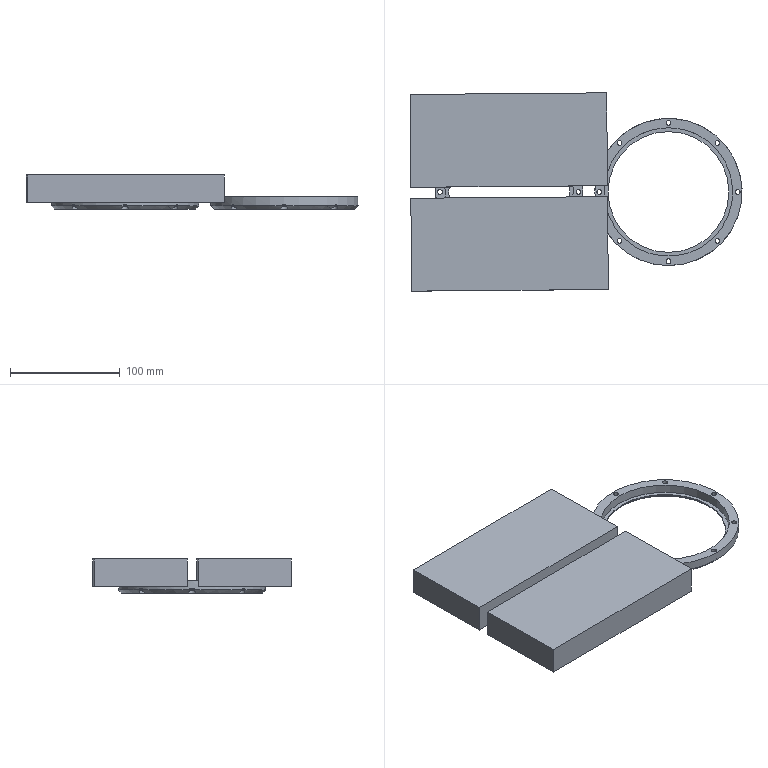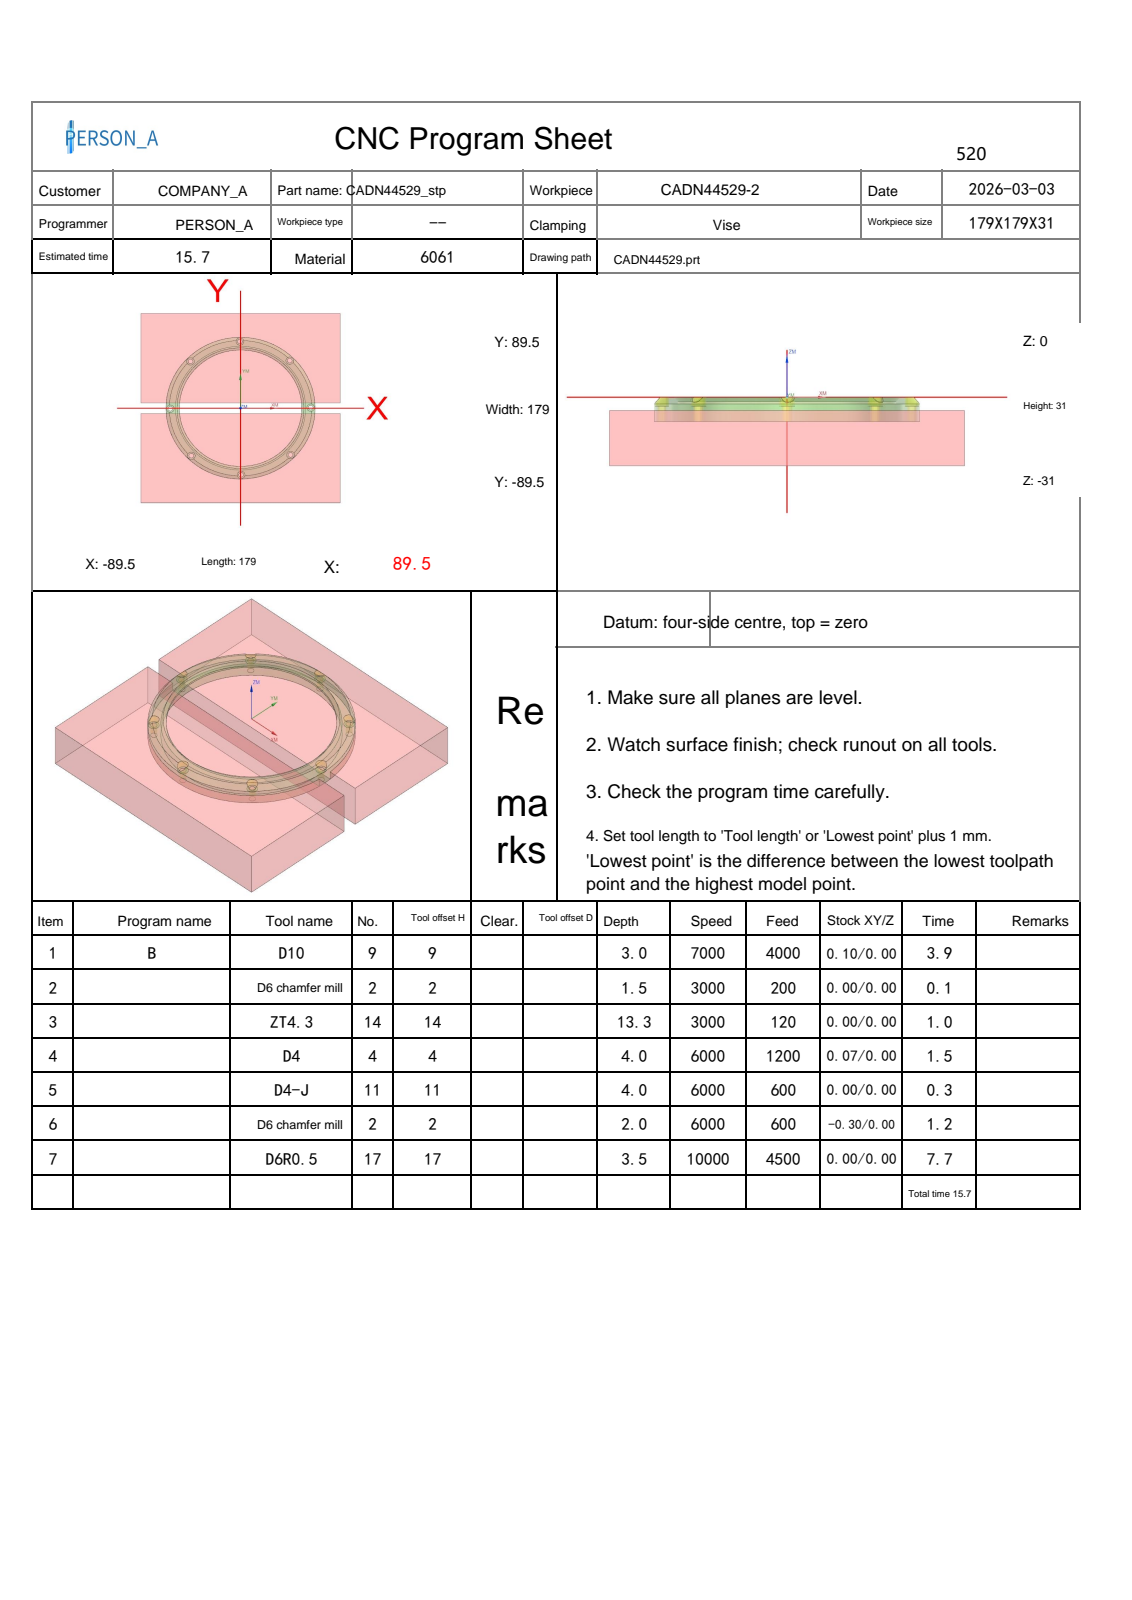NC program | NX | posted by the shop | part box 302.234 x 180.468 x 31 mm
Lines 21303 to 22985 of 75694, first 1471 of 1683 lines:
N2 T02 M06
(D6 chamfer mill  D=6. R=0. H=02 ce=0.00 di=0.00)
G00 G90 G54 X-44.913 Y44.179 M03 S3000
G43 H02 Z50.
M08
G98 G81 X-44.913 Y44.179 Z-1.5 R1. F200.
X-62.998 Y-.519
X-44.179 Y-44.913
X.519 Y-62.998
X44.913 Y-44.179
X62.998 Y.519
X44.179 Y44.913
X-.519 Y62.998
G80
G00 Z50.
G91 G28 Z0.0
M05
M09
G91 G28 Z0.0
M01
N3 T14 M06
(ZT4.3 D=4.3 DR_a=118 H=14)
G00 G90 G54 X-44.913 Y44.179 M03 S3000
G43 H14 Z50.
M08
G98 G83 X-44.913 Y44.179 Z-13.292 R1. F120. Q3.
X-62.998 Y-.519
X-44.179 Y-44.913
X.519 Y-62.998
X44.913 Y-44.179
X62.998 Y.519
X44.179 Y44.913
X-.519 Y62.998
G80
G00 Z50.
G91 G28 Z0.0
M05
M09
G91 G28 Z0.0
M01
N4 T04 M06
(D4  D=4. R=0. H=04 ce=0.07 di=0.00)
G00 G90 G54 X44.179 Y44.913 M03 S6000
G43 H04 Z50.
M08
Z.3
G03 X44.894 Y44.204 I.715 J.006 F1200.
X45.609 Y44.919 I0.0 J.715
G01 Y44.925
G03 X45.609 Y44.925 Z.1 I-1.43 J-.012
X45.609 Y44.925 Z-.1 I-1.43 J-.012
X45.609 Y44.925 Z-.3 I-1.43 J-.012
X45.609 Y44.925 Z-.5 I-1.43 J-.012
X45.609 Y44.925 Z-.7 I-1.43 J-.012
X45.609 Y44.925 Z-.9 I-1.43 J-.012
X45.609 Y44.925 Z-1.1 I-1.43 J-.012
X45.609 Y44.925 Z-1.3 I-1.43 J-.012
X45.609 Y44.925 Z-1.5 I-1.43 J-.012
X45.609 Y44.925 Z-1.7 I-1.43 J-.012
X45.609 Y44.925 Z-1.9 I-1.43 J-.012
X45.609 Y44.925 Z-2.1 I-1.43 J-.012
X45.609 Y44.925 Z-2.3 I-1.43 J-.012
X45.609 Y44.925 Z-2.5 I-1.43 J-.012
X45.609 Y44.925 Z-2.7 I-1.43 J-.012
X45.609 Y44.925 Z-2.9 I-1.43 J-.012
X45.609 Y44.925 Z-3.1 I-1.43 J-.012
X45.609 Y44.925 Z-3.3 I-1.43 J-.012
X45.609 Y44.925 Z-3.5 I-1.43 J-.012
X45.609 Y44.925 Z-3.7 I-1.43 J-.012
X45.609 Y44.925 Z-3.9 I-1.43 J-.012
X42.749 Y44.901 Z-4. I-1.43 J-.012
X44.179 Y43.483 I1.43 J.012
X45.609 Y44.913 I0.0 J1.43
X44.179 Y46.343 I-1.43 J0.0
X42.749 Y44.913 I0.0 J-1.43
G01 Y44.901
G03 X43.464 Y44.192 I.715 J.006
X44.179 Y44.907 I0.0 J.715
G01 Y44.913
G00 Z50.
X-.519 Y62.998
Z.3
G03 X.196 Y62.289 I.715 J.006
X.911 Y63.004 I0.0 J.715
G01 Y63.01
G03 X.911 Y63.01 Z.1 I-1.43 J-.012
X.911 Y63.01 Z-.1 I-1.43 J-.012
X.911 Y63.01 Z-.3 I-1.43 J-.012
X.911 Y63.01 Z-.5 I-1.43 J-.012
X.911 Y63.01 Z-.7 I-1.43 J-.012
X.911 Y63.01 Z-.9 I-1.43 J-.012
X.911 Y63.01 Z-1.1 I-1.43 J-.012
X.911 Y63.01 Z-1.3 I-1.43 J-.012
X.911 Y63.01 Z-1.5 I-1.43 J-.012
X.911 Y63.01 Z-1.7 I-1.43 J-.012
X.911 Y63.01 Z-1.9 I-1.43 J-.012
X.911 Y63.01 Z-2.1 I-1.43 J-.012
X.911 Y63.01 Z-2.3 I-1.43 J-.012
X.911 Y63.01 Z-2.5 I-1.43 J-.012
X.911 Y63.01 Z-2.7 I-1.43 J-.012
X.911 Y63.01 Z-2.9 I-1.43 J-.012
X.911 Y63.01 Z-3.1 I-1.43 J-.012
X.911 Y63.01 Z-3.3 I-1.43 J-.012
X.911 Y63.01 Z-3.5 I-1.43 J-.012
X.911 Y63.01 Z-3.7 I-1.43 J-.012
X.911 Y63.01 Z-3.9 I-1.43 J-.012
X-1.949 Y62.982 Z-4. I-1.43 J-.012
X-.519 Y61.568 I1.43 J.016
X.911 Y62.998 I0.0 J1.43
X-.519 Y64.428 I-1.43 J0.0
X-1.949 Y62.998 I0.0 J-1.43
G01 Y62.982
G03 X-1.234 Y62.275 I.715 J.008
X-.519 Y62.99 I0.0 J.715
G01 Y62.998
G00 Z50.
X-44.913 Y44.179
Z.3
G03 X-44.198 Y43.47 I.715 J.006
X-43.483 Y44.185 I0.0 J.715
G01 Y44.191
G03 X-43.483 Y44.191 Z.1 I-1.43 J-.012
X-43.483 Y44.191 Z-.1 I-1.43 J-.012
X-43.483 Y44.191 Z-.3 I-1.43 J-.012
X-43.483 Y44.191 Z-.5 I-1.43 J-.012
X-43.483 Y44.191 Z-.7 I-1.43 J-.012
X-43.483 Y44.191 Z-.9 I-1.43 J-.012
X-43.483 Y44.191 Z-1.1 I-1.43 J-.012
X-43.483 Y44.191 Z-1.3 I-1.43 J-.012
X-43.483 Y44.191 Z-1.5 I-1.43 J-.012
X-43.483 Y44.191 Z-1.7 I-1.43 J-.012
X-43.483 Y44.191 Z-1.9 I-1.43 J-.012
X-43.483 Y44.191 Z-2.1 I-1.43 J-.012
X-43.483 Y44.191 Z-2.3 I-1.43 J-.012
X-43.483 Y44.191 Z-2.5 I-1.43 J-.012
X-43.483 Y44.191 Z-2.7 I-1.43 J-.012
X-43.483 Y44.191 Z-2.9 I-1.43 J-.012
X-43.483 Y44.191 Z-3.1 I-1.43 J-.012
X-43.483 Y44.191 Z-3.3 I-1.43 J-.012
X-43.483 Y44.191 Z-3.5 I-1.43 J-.012
X-43.483 Y44.191 Z-3.7 I-1.43 J-.012
X-43.483 Y44.191 Z-3.9 I-1.43 J-.012
X-46.343 Y44.167 Z-4. I-1.43 J-.012
X-44.913 Y42.749 I1.43 J.012
X-43.483 Y44.179 I0.0 J1.43
X-44.913 Y45.609 I-1.43 J0.0
X-46.343 Y44.179 I0.0 J-1.43
G01 Y44.167
G03 X-45.628 Y43.458 I.715 J.006
X-44.913 Y44.173 I0.0 J.715
G01 Y44.179
G00 Z50.
X-62.998 Y-.519
Z.3
G03 X-62.283 Y-1.228 I.715 J.006
X-61.568 Y-.513 I0.0 J.715
G01 Y-.507
G03 X-61.568 Y-.507 Z.1 I-1.43 J-.012
X-61.568 Y-.507 Z-.1 I-1.43 J-.012
X-61.568 Y-.507 Z-.3 I-1.43 J-.012
X-61.568 Y-.507 Z-.5 I-1.43 J-.012
X-61.568 Y-.507 Z-.7 I-1.43 J-.012
X-61.568 Y-.507 Z-.9 I-1.43 J-.012
X-61.568 Y-.507 Z-1.1 I-1.43 J-.012
X-61.568 Y-.507 Z-1.3 I-1.43 J-.012
X-61.568 Y-.507 Z-1.5 I-1.43 J-.012
X-61.568 Y-.507 Z-1.7 I-1.43 J-.012
X-61.568 Y-.507 Z-1.9 I-1.43 J-.012
X-61.568 Y-.507 Z-2.1 I-1.43 J-.012
X-61.568 Y-.507 Z-2.3 I-1.43 J-.012
X-61.568 Y-.507 Z-2.5 I-1.43 J-.012
X-61.568 Y-.507 Z-2.7 I-1.43 J-.012
X-61.568 Y-.507 Z-2.9 I-1.43 J-.012
X-61.568 Y-.507 Z-3.1 I-1.43 J-.012
X-61.568 Y-.507 Z-3.3 I-1.43 J-.012
X-61.568 Y-.507 Z-3.5 I-1.43 J-.012
X-61.568 Y-.507 Z-3.7 I-1.43 J-.012
X-61.568 Y-.507 Z-3.9 I-1.43 J-.012
X-64.428 Y-.531 Z-4. I-1.43 J-.012
X-62.998 Y-1.949 I1.43 J.012
X-61.568 Y-.519 I0.0 J1.43
X-62.998 Y.911 I-1.43 J0.0
X-64.428 Y-.519 I0.0 J-1.43
G01 Y-.531
G03 X-63.713 Y-1.24 I.715 J.006
X-62.998 Y-.525 I0.0 J.715
G01 Y-.519
G00 Z50.
X-44.179 Y-44.913
Z.3
G03 X-43.464 Y-45.622 I.715 J.006
X-42.749 Y-44.907 I0.0 J.715
G01 Y-44.901
G03 X-42.749 Y-44.901 Z.1 I-1.43 J-.012
X-42.749 Y-44.901 Z-.1 I-1.43 J-.012
X-42.749 Y-44.901 Z-.3 I-1.43 J-.012
X-42.749 Y-44.901 Z-.5 I-1.43 J-.012
X-42.749 Y-44.901 Z-.7 I-1.43 J-.012
X-42.749 Y-44.901 Z-.9 I-1.43 J-.012
X-42.749 Y-44.901 Z-1.1 I-1.43 J-.012
X-42.749 Y-44.901 Z-1.3 I-1.43 J-.012
X-42.749 Y-44.901 Z-1.5 I-1.43 J-.012
X-42.749 Y-44.901 Z-1.7 I-1.43 J-.012
X-42.749 Y-44.901 Z-1.9 I-1.43 J-.012
X-42.749 Y-44.901 Z-2.1 I-1.43 J-.012
X-42.749 Y-44.901 Z-2.3 I-1.43 J-.012
X-42.749 Y-44.901 Z-2.5 I-1.43 J-.012
X-42.749 Y-44.901 Z-2.7 I-1.43 J-.012
X-42.749 Y-44.901 Z-2.9 I-1.43 J-.012
X-42.749 Y-44.901 Z-3.1 I-1.43 J-.012
X-42.749 Y-44.901 Z-3.3 I-1.43 J-.012
X-42.749 Y-44.901 Z-3.5 I-1.43 J-.012
X-42.749 Y-44.901 Z-3.7 I-1.43 J-.012
X-42.749 Y-44.901 Z-3.9 I-1.43 J-.012
X-45.609 Y-44.925 Z-4. I-1.43 J-.012
X-44.179 Y-46.343 I1.43 J.012
X-42.749 Y-44.913 I0.0 J1.43
X-44.179 Y-43.483 I-1.43 J0.0
X-45.609 Y-44.913 I0.0 J-1.43
G01 Y-44.925
G03 X-44.894 Y-45.634 I.715 J.006
X-44.179 Y-44.919 I0.0 J.715
G01 Y-44.913
G00 Z50.
X.519 Y-62.998
Z.3
G03 X1.234 Y-63.707 I.715 J.006
X1.949 Y-62.992 I0.0 J.715
G01 Y-62.986
G03 X1.949 Y-62.986 Z.1 I-1.43 J-.012
X1.949 Y-62.986 Z-.1 I-1.43 J-.012
X1.949 Y-62.986 Z-.3 I-1.43 J-.012
X1.949 Y-62.986 Z-.5 I-1.43 J-.012
X1.949 Y-62.986 Z-.7 I-1.43 J-.012
X1.949 Y-62.986 Z-.9 I-1.43 J-.012
X1.949 Y-62.986 Z-1.1 I-1.43 J-.012
X1.949 Y-62.986 Z-1.3 I-1.43 J-.012
X1.949 Y-62.986 Z-1.5 I-1.43 J-.012
X1.949 Y-62.986 Z-1.7 I-1.43 J-.012
X1.949 Y-62.986 Z-1.9 I-1.43 J-.012
X1.949 Y-62.986 Z-2.1 I-1.43 J-.012
X1.949 Y-62.986 Z-2.3 I-1.43 J-.012
X1.949 Y-62.986 Z-2.5 I-1.43 J-.012
X1.949 Y-62.986 Z-2.7 I-1.43 J-.012
X1.949 Y-62.986 Z-2.9 I-1.43 J-.012
X1.949 Y-62.986 Z-3.1 I-1.43 J-.012
X1.949 Y-62.986 Z-3.3 I-1.43 J-.012
X1.949 Y-62.986 Z-3.5 I-1.43 J-.012
X1.949 Y-62.986 Z-3.7 I-1.43 J-.012
X1.949 Y-62.986 Z-3.9 I-1.43 J-.012
X-.911 Y-63.01 Z-4. I-1.43 J-.012
X.519 Y-64.428 I1.43 J.012
X1.949 Y-62.998 I0.0 J1.43
X.519 Y-61.568 I-1.43 J0.0
X-.911 Y-62.998 I0.0 J-1.43
G01 Y-63.01
G03 X-.196 Y-63.719 I.715 J.006
X.519 Y-63.004 I0.0 J.715
G01 Y-62.998
G00 Z50.
X44.913 Y-44.179
Z.3
G03 X45.628 Y-44.888 I.715 J.006
X46.343 Y-44.173 I0.0 J.715
G01 Y-44.167
G03 X46.343 Y-44.167 Z.1 I-1.43 J-.012
X46.343 Y-44.167 Z-.1 I-1.43 J-.012
X46.343 Y-44.167 Z-.3 I-1.43 J-.012
X46.343 Y-44.167 Z-.5 I-1.43 J-.012
X46.343 Y-44.167 Z-.7 I-1.43 J-.012
X46.343 Y-44.167 Z-.9 I-1.43 J-.012
X46.343 Y-44.167 Z-1.1 I-1.43 J-.012
X46.343 Y-44.167 Z-1.3 I-1.43 J-.012
X46.343 Y-44.167 Z-1.5 I-1.43 J-.012
X46.343 Y-44.167 Z-1.7 I-1.43 J-.012
X46.343 Y-44.167 Z-1.9 I-1.43 J-.012
X46.343 Y-44.167 Z-2.1 I-1.43 J-.012
X46.343 Y-44.167 Z-2.3 I-1.43 J-.012
X46.343 Y-44.167 Z-2.5 I-1.43 J-.012
X46.343 Y-44.167 Z-2.7 I-1.43 J-.012
X46.343 Y-44.167 Z-2.9 I-1.43 J-.012
X46.343 Y-44.167 Z-3.1 I-1.43 J-.012
X46.343 Y-44.167 Z-3.3 I-1.43 J-.012
X46.343 Y-44.167 Z-3.5 I-1.43 J-.012
X46.343 Y-44.167 Z-3.7 I-1.43 J-.012
X46.343 Y-44.167 Z-3.9 I-1.43 J-.012
X43.483 Y-44.191 Z-4. I-1.43 J-.012
X44.913 Y-45.609 I1.43 J.012
X46.343 Y-44.179 I0.0 J1.43
X44.913 Y-42.749 I-1.43 J0.0
X43.483 Y-44.179 I0.0 J-1.43
G01 Y-44.191
G03 X44.198 Y-44.9 I.715 J.006
X44.913 Y-44.185 I0.0 J.715
G01 Y-44.179
G00 Z50.
X62.998 Y.519
Z.3
G03 X63.713 Y-.19 I.715 J.006
X64.428 Y.525 I0.0 J.715
G01 Y.531
G03 X64.428 Y.531 Z.1 I-1.43 J-.012
X64.428 Y.531 Z-.1 I-1.43 J-.012
X64.428 Y.531 Z-.3 I-1.43 J-.012
X64.428 Y.531 Z-.5 I-1.43 J-.012
X64.428 Y.531 Z-.7 I-1.43 J-.012
X64.428 Y.531 Z-.9 I-1.43 J-.012
X64.428 Y.531 Z-1.1 I-1.43 J-.012
X64.428 Y.531 Z-1.3 I-1.43 J-.012
X64.428 Y.531 Z-1.5 I-1.43 J-.012
X64.428 Y.531 Z-1.7 I-1.43 J-.012
X64.428 Y.531 Z-1.9 I-1.43 J-.012
X64.428 Y.531 Z-2.1 I-1.43 J-.012
X64.428 Y.531 Z-2.3 I-1.43 J-.012
X64.428 Y.531 Z-2.5 I-1.43 J-.012
X64.428 Y.531 Z-2.7 I-1.43 J-.012
X64.428 Y.531 Z-2.9 I-1.43 J-.012
X64.428 Y.531 Z-3.1 I-1.43 J-.012
X64.428 Y.531 Z-3.3 I-1.43 J-.012
X64.428 Y.531 Z-3.5 I-1.43 J-.012
X64.428 Y.531 Z-3.7 I-1.43 J-.012
X64.428 Y.531 Z-3.9 I-1.43 J-.012
X61.568 Y.503 Z-4. I-1.43 J-.012
X62.998 Y-.911 I1.43 J.016
X64.428 Y.519 I0.0 J1.43
X62.998 Y1.949 I-1.43 J0.0
X61.568 Y.519 I0.0 J-1.43
G01 Y.503
G03 X62.283 Y-.204 I.715 J.008
X62.998 Y.511 I0.0 J.715
G01 Y.519
G00 Z50.
G91 G28 Z0.0
M05
M09
G91 G28 Z0.0
M01
N5 T11 M06
(D4-J  D=4. R=0. H=11 ce=0.00 di=0.00)
G00 G90 G54 X44.179 Y44.913 M03 S6000
G43 H11 Z50.
M08
Z-4.
G01 X45.268 Y44.61 F600.
X45.355 Y44.598
G03 X45.679 Y44.923 I0.0 J.324
G01 Y44.926
G03 X44.179 Y46.413 I-1.5 J-.012
X42.679 Y44.913 I0.0 J-1.5
X44.179 Y43.413 I1.5 J0.0
X45.679 Y44.913 I0.0 J1.5
X45.593 Y45.416 I-1.5 J0.0
X45.287 Y45.631 I-.306 J-.109
X45.098 Y45.571 I0.0 J-.324
G01 X44.179 Y44.913
G00 Z50.
X-.519 Y62.998
Z-4.
G01 X.57 Y62.695
X.657 Y62.683
G03 X.981 Y63.008 I0.0 J.324
G01 Y63.01
G03 X-.519 Y64.498 I-1.5 J-.012
X-2.019 Y62.998 I0.0 J-1.5
X-.519 Y61.498 I1.5 J0.0
X.981 Y62.998 I0.0 J1.5
X.894 Y63.5 I-1.5 J0.0
X.589 Y63.716 I-.306 J-.109
X.4 Y63.655 I0.0 J-.324
G01 X-.519 Y62.998
G00 Z50.
X-44.913 Y44.179
Z-4.
G01 X-43.825 Y43.876
X-43.738 Y43.865
G03 X-43.413 Y44.189 I0.0 J.324
G01 Y44.192
G03 X-44.913 Y45.679 I-1.5 J-.012
X-46.413 Y44.179 I0.0 J-1.5
X-44.913 Y42.679 I1.5 J0.0
X-43.413 Y44.179 I0.0 J1.5
X-43.5 Y44.682 I-1.5 J0.0
X-43.805 Y44.897 I-.306 J-.109
X-43.994 Y44.837 I0.0 J-.324
G01 X-44.913 Y44.179
G00 Z50.
X-62.998 Y-.519
Z-4.
G01 X-61.909 Y-.822
X-61.822 Y-.834
G03 X-61.498 Y-.509 I0.0 J.324
G01 Y-.507
G03 X-62.998 Y.981 I-1.5 J-.012
X-64.498 Y-.519 I0.0 J-1.5
X-62.998 Y-2.019 I1.5 J0.0
X-61.498 Y-.519 I0.0 J1.5
X-61.585 Y-.017 I-1.5 J0.0
X-61.89 Y.199 I-.306 J-.109
X-62.079 Y.139 I0.0 J-.324
G01 X-62.998 Y-.519
G00 Z50.
X-44.179 Y-44.913
Z-4.
G01 X-43.091 Y-45.216
X-43.004 Y-45.228
G03 X-42.679 Y-44.903 I0.0 J.324
G01 Y-44.901
G03 X-44.179 Y-43.413 I-1.5 J-.012
X-45.679 Y-44.913 I0.0 J-1.5
X-44.179 Y-46.413 I1.5 J0.0
X-42.679 Y-44.913 I0.0 J1.5
X-42.766 Y-44.411 I-1.5 J0.0
X-43.072 Y-44.195 I-.306 J-.109
X-43.26 Y-44.256 I0.0 J-.324
G01 X-44.179 Y-44.913
G00 Z50.
X.519 Y-62.998
Z-4.
G01 X1.608 Y-63.301
X1.695 Y-63.313
G03 X2.019 Y-62.988 I0.0 J.324
G01 Y-62.986
G03 X.519 Y-61.498 I-1.5 J-.012
X-.981 Y-62.998 I0.0 J-1.5
X.519 Y-64.498 I1.5 J0.0
X2.019 Y-62.998 I0.0 J1.5
X1.932 Y-62.495 I-1.5 J0.0
X1.627 Y-62.28 I-.306 J-.109
X1.438 Y-62.34 I0.0 J-.324
G01 X.519 Y-62.998
G00 Z50.
X44.913 Y-44.179
Z-4.
G01 X46.002 Y-44.482
X46.089 Y-44.494
G03 X46.413 Y-44.17 I0.0 J.324
G01 Y-44.167
G03 X44.913 Y-42.679 I-1.5 J-.012
X43.413 Y-44.179 I0.0 J-1.5
X44.913 Y-45.679 I1.5 J0.0
X46.413 Y-44.179 I0.0 J1.5
X46.327 Y-43.677 I-1.5 J0.0
X46.021 Y-43.461 I-.306 J-.109
X45.832 Y-43.522 I0.0 J-.324
G01 X44.913 Y-44.179
G00 Z50.
X62.998 Y.519
Z-4.
G01 X64.087 Y.216
X64.173 Y.204
G03 X64.498 Y.529 I0.0 J.324
G01 Y.531
G03 X62.998 Y2.019 I-1.5 J-.012
X61.498 Y.519 I0.0 J-1.5
X62.998 Y-.981 I1.5 J0.0
X64.498 Y.519 I0.0 J1.5
X64.411 Y1.021 I-1.5 J0.0
X64.106 Y1.237 I-.306 J-.109
X63.917 Y1.177 I0.0 J-.324
G01 X62.998 Y.519
G00 Z50.
G91 G28 Z0.0
M05
M09
G91 G28 Z0.0
M01
N6 T02 M06
(D6 chamfer mill  D=6. R=0. H=02 ce=-0.30 di=0.00)
G00 G90 G54 X1.534 Y-62.2 M03 S6000
G43 H02 Z50.
M08
Z.5
G01 X2.13 Y-62.195 Z.479 F600.
X2.07 Y-62.075 Z.474
X1.864 Y-61.794 Z.462
X1.607 Y-61.558 Z.45
X1.31 Y-61.375 Z.438
X.983 Y-61.253 Z.426
X.638 Y-61.197 Z.413
X.37 Y-61.199 Z.404
X.027 Y-61.261 Z.392
X-.298 Y-61.388 Z.38
X-.593 Y-61.576 Z.368
X-.845 Y-61.816 Z.355
X-1.047 Y-62.101 Z.343
X-1.105 Y-62.222 Z.338
X2.13 Y-62.195 Z.226
X2.07 Y-62.075 Z.221
X1.864 Y-61.794 Z.209
X1.607 Y-61.558 Z.196
X1.31 Y-61.375 Z.184
X.983 Y-61.253 Z.172
X.638 Y-61.197 Z.16
X.37 Y-61.199 Z.151
X.027 Y-61.261 Z.138
X-.298 Y-61.388 Z.126
X-.593 Y-61.576 Z.114
X-.845 Y-61.816 Z.102
X-1.047 Y-62.101 Z.09
X-1.105 Y-62.222 Z.085
X2.13 Y-62.195 Z-.028
X2.07 Y-62.075 Z-.033
X1.864 Y-61.794 Z-.045
X1.607 Y-61.558 Z-.057
X1.31 Y-61.375 Z-.069
X.983 Y-61.253 Z-.081
X.638 Y-61.197 Z-.094
X.37 Y-61.199 Z-.103
X.027 Y-61.261 Z-.115
X-.298 Y-61.388 Z-.127
X-.593 Y-61.576 Z-.14
X-.845 Y-61.816 Z-.152
X-1.047 Y-62.101 Z-.164
X-1.105 Y-62.222 Z-.169
X2.13 Y-62.195 Z-.282
X2.07 Y-62.075 Z-.286
X1.864 Y-61.794 Z-.298
X1.607 Y-61.558 Z-.311
X1.31 Y-61.375 Z-.323
X.983 Y-61.253 Z-.335
X.638 Y-61.197 Z-.347
X.37 Y-61.199 Z-.357
X.027 Y-61.261 Z-.369
X-.298 Y-61.388 Z-.381
X-.593 Y-61.576 Z-.393
X-.845 Y-61.816 Z-.405
X-1.047 Y-62.101 Z-.418
X-1.105 Y-62.222 Z-.422
X2.13 Y-62.195 Z-.535
X2.07 Y-62.075 Z-.54
X1.864 Y-61.794 Z-.552
X1.607 Y-61.558 Z-.564
X1.31 Y-61.375 Z-.576
X.983 Y-61.253 Z-.589
X.638 Y-61.197 Z-.601
X.37 Y-61.199 Z-.61
X.027 Y-61.261 Z-.622
X-.298 Y-61.388 Z-.635
X-.593 Y-61.576 Z-.647
X-.845 Y-61.816 Z-.659
X-1.047 Y-62.101 Z-.671
X-1.105 Y-62.222 Z-.676
X2.13 Y-62.195 Z-.789
X2.07 Y-62.075 Z-.793
X1.864 Y-61.794 Z-.806
X1.607 Y-61.558 Z-.818
X1.31 Y-61.375 Z-.83
X.983 Y-61.253 Z-.842
X.638 Y-61.197 Z-.854
X.37 Y-61.199 Z-.864
X.027 Y-61.261 Z-.876
X-.298 Y-61.388 Z-.888
X-.593 Y-61.576 Z-.9
X-.845 Y-61.816 Z-.912
X-1.047 Y-62.101 Z-.925
X-1.105 Y-62.222 Z-.929
X2.13 Y-62.195 Z-1.042
X2.07 Y-62.075 Z-1.047
X1.864 Y-61.794 Z-1.059
X1.607 Y-61.558 Z-1.071
X1.31 Y-61.375 Z-1.084
X.983 Y-61.253 Z-1.096
X.638 Y-61.197 Z-1.108
X.37 Y-61.199 Z-1.117
X.027 Y-61.261 Z-1.129
X-.298 Y-61.388 Z-1.142
X-.593 Y-61.576 Z-1.154
X-.845 Y-61.816 Z-1.166
X-1.047 Y-62.101 Z-1.178
X-1.105 Y-62.222 Z-1.183
X2.13 Y-62.195 Z-1.296
X2.07 Y-62.075 Z-1.301
X1.864 Y-61.794 Z-1.313
X1.607 Y-61.558 Z-1.325
X1.31 Y-61.375 Z-1.337
X.983 Y-61.253 Z-1.349
X.638 Y-61.197 Z-1.361
X.37 Y-61.199 Z-1.371
X.027 Y-61.261 Z-1.383
X-.298 Y-61.388 Z-1.395
X-.593 Y-61.576 Z-1.407
X-.845 Y-61.816 Z-1.42
X-1.047 Y-62.101 Z-1.432
X-1.105 Y-62.222 Z-1.436
X2.13 Y-62.195 Z-1.549
X2.07 Y-62.075 Z-1.554
X1.864 Y-61.794 Z-1.566
X1.607 Y-61.558 Z-1.579
X1.31 Y-61.375 Z-1.591
X.983 Y-61.253 Z-1.603
X.638 Y-61.197 Z-1.615
X.37 Y-61.199 Z-1.624
X.027 Y-61.261 Z-1.637
X-.298 Y-61.388 Z-1.649
X-.593 Y-61.576 Z-1.661
X-.845 Y-61.816 Z-1.673
X-1.047 Y-62.101 Z-1.685
X-1.105 Y-62.222 Z-1.69
X2.13 Y-62.195 Z-1.803
X2.07 Y-62.075 Z-1.808
X1.864 Y-61.794 Z-1.82
X1.607 Y-61.558 Z-1.832
X1.31 Y-61.375 Z-1.844
X.983 Y-61.253 Z-1.856
X.638 Y-61.197 Z-1.869
X.37 Y-61.199 Z-1.878
X.027 Y-61.261 Z-1.89
X-.298 Y-61.388 Z-1.902
X-.593 Y-61.576 Z-1.915
X-.845 Y-61.816 Z-1.927
X-1.047 Y-62.101 Z-1.939
X-1.105 Y-62.222 Z-1.944
X.512 Y-62.209 Z-2.
X2.13 Y-62.195
G03 X.519 Y-61.198 I-1.611 J-.803
X-1.105 Y-62.222 I0.0 J-1.8
G01 X.512 Y-62.209
G03 X1.569 Y-61.76 I-.012 J1.5
G01 Z-1.5
G00 Z50.
X-42.895 Y-45.07
Z.5
G01 X-42.472 Y-45.485 Z.479
X-42.43 Y-45.358 Z.475
X-42.377 Y-45.013 Z.462
X-42.392 Y-44.664 Z.45
X-42.473 Y-44.325 Z.438
X-42.618 Y-44.008 Z.426
X-42.821 Y-43.724 Z.414
X-43.013 Y-43.536 Z.404
X-43.3 Y-43.337 Z.392
X-43.619 Y-43.197 Z.38
X-43.96 Y-43.122 Z.368
X-44.309 Y-43.113 Z.355
X-44.653 Y-43.171 Z.343
X-44.779 Y-43.216 Z.339
X-42.472 Y-45.485 Z.226
X-42.43 Y-45.358 Z.221
X-42.377 Y-45.013 Z.209
X-42.392 Y-44.664 Z.197
X-42.473 Y-44.325 Z.184
X-42.618 Y-44.008 Z.172
X-42.821 Y-43.724 Z.16
X-43.013 Y-43.536 Z.151
X-43.3 Y-43.337 Z.138
X-43.619 Y-43.197 Z.126
X-43.96 Y-43.122 Z.114
X-44.309 Y-43.113 Z.102
X-44.653 Y-43.171 Z.09
X-44.779 Y-43.216 Z.085
X-42.472 Y-45.485 Z-.028
X-42.43 Y-45.358 Z-.033
X-42.377 Y-45.013 Z-.045
X-42.392 Y-44.664 Z-.057
X-42.473 Y-44.325 Z-.069
X-42.618 Y-44.008 Z-.081
X-42.821 Y-43.724 Z-.094
X-43.013 Y-43.536 Z-.103
X-43.3 Y-43.337 Z-.115
X-43.619 Y-43.197 Z-.127
X-43.96 Y-43.122 Z-.139
X-44.309 Y-43.113 Z-.152
X-44.653 Y-43.171 Z-.164
X-44.779 Y-43.216 Z-.169
X-42.472 Y-45.485 Z-.282
X-42.43 Y-45.358 Z-.286
X-42.377 Y-45.013 Z-.298
X-42.392 Y-44.664 Z-.311
X-42.473 Y-44.325 Z-.323
X-42.618 Y-44.008 Z-.335
X-42.821 Y-43.724 Z-.347
X-43.013 Y-43.536 Z-.357
X-43.3 Y-43.337 Z-.369
X-43.619 Y-43.197 Z-.381
X-43.96 Y-43.122 Z-.393
X-44.309 Y-43.113 Z-.405
X-44.653 Y-43.171 Z-.417
X-44.779 Y-43.216 Z-.422
X-42.472 Y-45.485 Z-.535
X-42.43 Y-45.358 Z-.54
X-42.377 Y-45.013 Z-.552
X-42.392 Y-44.664 Z-.564
X-42.473 Y-44.325 Z-.576
X-42.618 Y-44.008 Z-.589
X-42.821 Y-43.724 Z-.601
X-43.013 Y-43.536 Z-.61
X-43.3 Y-43.337 Z-.622
X-43.619 Y-43.197 Z-.634
X-43.96 Y-43.122 Z-.647
X-44.309 Y-43.113 Z-.659
X-44.653 Y-43.171 Z-.671
X-44.779 Y-43.216 Z-.676
X-42.472 Y-45.485 Z-.789
X-42.43 Y-45.358 Z-.793
X-42.377 Y-45.013 Z-.806
X-42.392 Y-44.664 Z-.818
X-42.473 Y-44.325 Z-.83
X-42.618 Y-44.008 Z-.842
X-42.821 Y-43.724 Z-.854
X-43.013 Y-43.536 Z-.864
X-43.3 Y-43.337 Z-.876
X-43.619 Y-43.197 Z-.888
X-43.96 Y-43.122 Z-.9
X-44.309 Y-43.113 Z-.912
X-44.653 Y-43.171 Z-.925
X-44.779 Y-43.216 Z-.929
X-42.472 Y-45.485 Z-1.042
X-42.43 Y-45.358 Z-1.047
X-42.377 Y-45.013 Z-1.059
X-42.392 Y-44.664 Z-1.071
X-42.473 Y-44.325 Z-1.084
X-42.618 Y-44.008 Z-1.096
X-42.821 Y-43.724 Z-1.108
X-43.013 Y-43.536 Z-1.117
X-43.3 Y-43.337 Z-1.129
X-43.619 Y-43.197 Z-1.142
X-43.96 Y-43.122 Z-1.154
X-44.309 Y-43.113 Z-1.166
X-44.653 Y-43.171 Z-1.178
X-44.779 Y-43.216 Z-1.183
X-42.472 Y-45.485 Z-1.296
X-42.43 Y-45.358 Z-1.301
X-42.377 Y-45.013 Z-1.313
X-42.392 Y-44.664 Z-1.325
X-42.473 Y-44.325 Z-1.337
X-42.618 Y-44.008 Z-1.349
X-42.821 Y-43.724 Z-1.361
X-43.013 Y-43.536 Z-1.371
X-43.3 Y-43.337 Z-1.383
X-43.619 Y-43.197 Z-1.395
X-43.96 Y-43.122 Z-1.407
X-44.309 Y-43.113 Z-1.42
X-44.653 Y-43.171 Z-1.432
X-44.779 Y-43.216 Z-1.436
X-42.472 Y-45.485 Z-1.549
X-42.43 Y-45.358 Z-1.554
X-42.377 Y-45.013 Z-1.566
X-42.392 Y-44.664 Z-1.578
X-42.473 Y-44.325 Z-1.591
X-42.618 Y-44.008 Z-1.603
X-42.821 Y-43.724 Z-1.615
X-43.013 Y-43.536 Z-1.624
X-43.3 Y-43.337 Z-1.637
X-43.619 Y-43.197 Z-1.649
X-43.96 Y-43.122 Z-1.661
X-44.309 Y-43.113 Z-1.673
X-44.653 Y-43.171 Z-1.685
X-44.779 Y-43.216 Z-1.69
X-42.472 Y-45.485 Z-1.803
X-42.43 Y-45.358 Z-1.808
X-42.377 Y-45.013 Z-1.82
X-42.392 Y-44.664 Z-1.832
X-42.473 Y-44.325 Z-1.844
X-42.618 Y-44.008 Z-1.856
X-42.821 Y-43.724 Z-1.869
X-43.013 Y-43.536 Z-1.878
X-43.3 Y-43.337 Z-1.89
X-43.619 Y-43.197 Z-1.902
X-43.96 Y-43.122 Z-1.915
X-44.309 Y-43.113 Z-1.927
X-44.653 Y-43.171 Z-1.939
X-44.779 Y-43.216 Z-1.944
X-43.626 Y-44.351 Z-2.
X-42.472 Y-45.485
G03 X-42.379 Y-44.913 I-1.707 J.572
X-44.179 Y-43.113 I-1.8 J0.0
X-44.779 Y-43.216 I0.0 J-1.8
G01 X-43.626 Y-44.351
G03 X-42.574 Y-44.781 I1.052 J1.069
G01 X-42.562
Z-1.5
G00 Z50.
X-62.2 Y-1.533
Z.5
G01 X-62.195 Y-2.13 Z.479
X-62.075 Y-2.07 Z.474
X-61.794 Y-1.864 Z.462
X-61.558 Y-1.607 Z.45
X-61.375 Y-1.31 Z.438
X-61.253 Y-.983 Z.426
X-61.197 Y-.638 Z.413
X-61.199 Y-.37 Z.404
X-61.261 Y-.027 Z.392
X-61.388 Y.298 Z.38
X-61.576 Y.593 Z.368
X-61.816 Y.845 Z.355
X-62.101 Y1.047 Z.343
X-62.222 Y1.105 Z.338
X-62.195 Y-2.13 Z.225
X-62.075 Y-2.07 Z.221
X-61.794 Y-1.864 Z.209
X-61.558 Y-1.607 Z.196
X-61.375 Y-1.31 Z.184
X-61.253 Y-.983 Z.172
X-61.197 Y-.638 Z.16
X-61.199 Y-.37 Z.151
X-61.261 Y-.027 Z.138
X-61.388 Y.298 Z.126
X-61.576 Y.593 Z.114
X-61.816 Y.845 Z.102
X-62.101 Y1.047 Z.09
X-62.222 Y1.105 Z.085
X-62.195 Y-2.13 Z-.028
X-62.075 Y-2.07 Z-.033
X-61.794 Y-1.864 Z-.045
X-61.558 Y-1.607 Z-.057
X-61.375 Y-1.31 Z-.069
X-61.253 Y-.983 Z-.082
X-61.197 Y-.638 Z-.094
X-61.199 Y-.37 Z-.103
X-61.261 Y-.027 Z-.115
X-61.388 Y.298 Z-.127
X-61.576 Y.593 Z-.14
X-61.816 Y.845 Z-.152
X-62.101 Y1.047 Z-.164
X-62.222 Y1.105 Z-.169
X-62.195 Y-2.13 Z-.282
X-62.075 Y-2.07 Z-.286
X-61.794 Y-1.864 Z-.299
X-61.558 Y-1.607 Z-.311
X-61.375 Y-1.31 Z-.323
X-61.253 Y-.983 Z-.335
X-61.197 Y-.638 Z-.347
X-61.199 Y-.37 Z-.357
X-61.261 Y-.027 Z-.369
X-61.388 Y.298 Z-.381
X-61.576 Y.593 Z-.393
X-61.816 Y.845 Z-.405
X-62.101 Y1.047 Z-.418
X-62.222 Y1.105 Z-.422
X-62.195 Y-2.13 Z-.535
X-62.075 Y-2.07 Z-.54
X-61.794 Y-1.864 Z-.552
X-61.558 Y-1.607 Z-.564
X-61.375 Y-1.31 Z-.576
X-61.253 Y-.983 Z-.589
X-61.197 Y-.638 Z-.601
X-61.199 Y-.37 Z-.61
X-61.261 Y-.027 Z-.622
X-61.388 Y.298 Z-.635
X-61.576 Y.593 Z-.647
X-61.816 Y.845 Z-.659
X-62.101 Y1.047 Z-.671
X-62.222 Y1.105 Z-.676
X-62.195 Y-2.13 Z-.789
X-62.075 Y-2.07 Z-.793
X-61.794 Y-1.864 Z-.806
X-61.558 Y-1.607 Z-.818
X-61.375 Y-1.31 Z-.83
X-61.253 Y-.983 Z-.842
X-61.197 Y-.638 Z-.854
X-61.199 Y-.37 Z-.864
X-61.261 Y-.027 Z-.876
X-61.388 Y.298 Z-.888
X-61.576 Y.593 Z-.9
X-61.816 Y.845 Z-.912
X-62.101 Y1.047 Z-.925
X-62.222 Y1.105 Z-.929
X-62.195 Y-2.13 Z-1.042
X-62.075 Y-2.07 Z-1.047
X-61.794 Y-1.864 Z-1.059
X-61.558 Y-1.607 Z-1.071
X-61.375 Y-1.31 Z-1.084
X-61.253 Y-.983 Z-1.096
X-61.197 Y-.638 Z-1.108
X-61.199 Y-.37 Z-1.117
X-61.261 Y-.027 Z-1.129
X-61.388 Y.298 Z-1.142
X-61.576 Y.593 Z-1.154
X-61.816 Y.845 Z-1.166
X-62.101 Y1.047 Z-1.178
X-62.222 Y1.105 Z-1.183
X-62.195 Y-2.13 Z-1.296
X-62.075 Y-2.07 Z-1.301
X-61.794 Y-1.864 Z-1.313
X-61.558 Y-1.607 Z-1.325
X-61.375 Y-1.31 Z-1.337
X-61.253 Y-.983 Z-1.349
X-61.197 Y-.638 Z-1.362
X-61.199 Y-.37 Z-1.371
X-61.261 Y-.027 Z-1.383
X-61.388 Y.298 Z-1.395
X-61.576 Y.593 Z-1.407
X-61.816 Y.845 Z-1.42
X-62.101 Y1.047 Z-1.432
X-62.222 Y1.105 Z-1.436
X-62.195 Y-2.13 Z-1.549
X-62.075 Y-2.07 Z-1.554
X-61.794 Y-1.864 Z-1.566
X-61.558 Y-1.607 Z-1.579
X-61.375 Y-1.31 Z-1.591
X-61.253 Y-.983 Z-1.603
X-61.197 Y-.638 Z-1.615
X-61.199 Y-.37 Z-1.624
X-61.261 Y-.027 Z-1.637
X-61.388 Y.298 Z-1.649
X-61.576 Y.593 Z-1.661
X-61.816 Y.845 Z-1.673
X-62.101 Y1.047 Z-1.685
X-62.222 Y1.105 Z-1.69
X-62.195 Y-2.13 Z-1.803
X-62.075 Y-2.07 Z-1.808
X-61.794 Y-1.864 Z-1.82
X-61.558 Y-1.607 Z-1.832
X-61.375 Y-1.31 Z-1.844
X-61.253 Y-.983 Z-1.856
X-61.197 Y-.638 Z-1.869
X-61.199 Y-.37 Z-1.878
X-61.261 Y-.027 Z-1.89
X-61.388 Y.298 Z-1.902
X-61.576 Y.593 Z-1.915
X-61.816 Y.845 Z-1.927
X-62.101 Y1.047 Z-1.939
X-62.222 Y1.105 Z-1.944
X-62.209 Y-.512 Z-2.
X-62.195 Y-2.13
G03 X-61.198 Y-.519 I-.803 J1.611
X-62.222 Y1.105 I-1.8 J0.0
G01 X-62.209 Y-.512
G03 X-61.76 Y-1.569 I1.5 J.012
G01 Z-1.5
G00 Z50.
X-45.068 Y42.896
Z.5
G01 X-45.485 Y42.472 Z.479
X-45.358 Y42.43 Z.474
X-45.013 Y42.377 Z.462
X-44.664 Y42.392 Z.45
X-44.325 Y42.473 Z.438
X-44.008 Y42.618 Z.426
X-43.724 Y42.821 Z.414
X-43.536 Y43.013 Z.404
X-43.337 Y43.299 Z.392
X-43.197 Y43.619 Z.38
X-43.122 Y43.96 Z.368
X-43.113 Y44.308 Z.355
X-43.171 Y44.652 Z.343
X-43.216 Y44.779 Z.339
X-45.485 Y42.472 Z.226
X-45.358 Y42.43 Z.221
X-45.013 Y42.377 Z.209
X-44.664 Y42.392 Z.197
X-44.325 Y42.473 Z.184
X-44.008 Y42.618 Z.172
X-43.724 Y42.821 Z.16
X-43.536 Y43.013 Z.151
X-43.337 Y43.299 Z.138
X-43.197 Y43.619 Z.126
X-43.122 Y43.96 Z.114
X-43.113 Y44.308 Z.102
X-43.171 Y44.652 Z.09
X-43.216 Y44.779 Z.085
X-45.485 Y42.472 Z-.028
X-45.358 Y42.43 Z-.033
X-45.013 Y42.377 Z-.045
X-44.664 Y42.392 Z-.057
X-44.325 Y42.473 Z-.069
X-44.008 Y42.618 Z-.081
X-43.724 Y42.821 Z-.094
X-43.536 Y43.013 Z-.103
X-43.337 Y43.299 Z-.115
X-43.197 Y43.619 Z-.127
X-43.122 Y43.96 Z-.14
X-43.113 Y44.308 Z-.152
X-43.171 Y44.652 Z-.164
X-43.216 Y44.779 Z-.169
X-45.485 Y42.472 Z-.282
X-45.358 Y42.43 Z-.286
X-45.013 Y42.377 Z-.298
X-44.664 Y42.392 Z-.311
X-44.325 Y42.473 Z-.323
X-44.008 Y42.618 Z-.335
X-43.724 Y42.821 Z-.347
X-43.536 Y43.013 Z-.357
X-43.337 Y43.299 Z-.369
X-43.197 Y43.619 Z-.381
X-43.122 Y43.96 Z-.393
X-43.113 Y44.308 Z-.405
X-43.171 Y44.652 Z-.417
X-43.216 Y44.779 Z-.422
X-45.485 Y42.472 Z-.535
X-45.358 Y42.43 Z-.54
X-45.013 Y42.377 Z-.552
X-44.664 Y42.392 Z-.564
X-44.325 Y42.473 Z-.576
X-44.008 Y42.618 Z-.589
X-43.724 Y42.821 Z-.601
X-43.536 Y43.013 Z-.61
X-43.337 Y43.299 Z-.622
X-43.197 Y43.619 Z-.635
X-43.122 Y43.96 Z-.647
X-43.113 Y44.308 Z-.659
X-43.171 Y44.652 Z-.671
X-43.216 Y44.779 Z-.676
X-45.485 Y42.472 Z-.789
X-45.358 Y42.43 Z-.793
X-45.013 Y42.377 Z-.806
X-44.664 Y42.392 Z-.818
X-44.325 Y42.473 Z-.83
X-44.008 Y42.618 Z-.842
X-43.724 Y42.821 Z-.854
X-43.536 Y43.013 Z-.864
X-43.337 Y43.299 Z-.876
X-43.197 Y43.619 Z-.888
X-43.122 Y43.96 Z-.9
X-43.113 Y44.308 Z-.912
X-43.171 Y44.652 Z-.925
X-43.216 Y44.779 Z-.929
X-45.485 Y42.472 Z-1.042
X-45.358 Y42.43 Z-1.047
X-45.013 Y42.377 Z-1.059
X-44.664 Y42.392 Z-1.071
X-44.325 Y42.473 Z-1.084
X-44.008 Y42.618 Z-1.096
X-43.724 Y42.821 Z-1.108
X-43.536 Y43.013 Z-1.117
X-43.337 Y43.299 Z-1.129
X-43.197 Y43.619 Z-1.142
X-43.122 Y43.96 Z-1.154
X-43.113 Y44.308 Z-1.166
X-43.171 Y44.652 Z-1.178
X-43.216 Y44.779 Z-1.183
X-45.485 Y42.472 Z-1.296
X-45.358 Y42.43 Z-1.301
X-45.013 Y42.377 Z-1.313
X-44.664 Y42.392 Z-1.325
X-44.325 Y42.473 Z-1.337
X-44.008 Y42.618 Z-1.349
X-43.724 Y42.821 Z-1.361
X-43.536 Y43.013 Z-1.371
X-43.337 Y43.299 Z-1.383
X-43.197 Y43.619 Z-1.395
X-43.122 Y43.96 Z-1.407
X-43.113 Y44.308 Z-1.42
X-43.171 Y44.652 Z-1.432
X-43.216 Y44.779 Z-1.436
X-45.485 Y42.472 Z-1.549
X-45.358 Y42.43 Z-1.554
X-45.013 Y42.377 Z-1.566
X-44.664 Y42.392 Z-1.579
X-44.325 Y42.473 Z-1.591
X-44.008 Y42.618 Z-1.603
X-43.724 Y42.821 Z-1.615
X-43.536 Y43.013 Z-1.624
X-43.337 Y43.299 Z-1.637
X-43.197 Y43.619 Z-1.649
X-43.122 Y43.96 Z-1.661
X-43.113 Y44.308 Z-1.673
X-43.171 Y44.652 Z-1.685
X-43.216 Y44.779 Z-1.69
X-45.485 Y42.472 Z-1.803
X-45.358 Y42.43 Z-1.808
X-45.013 Y42.377 Z-1.82
X-44.664 Y42.392 Z-1.832
X-44.325 Y42.473 Z-1.844
X-44.008 Y42.618 Z-1.856
X-43.724 Y42.821 Z-1.869
X-43.536 Y43.013 Z-1.878
X-43.337 Y43.299 Z-1.89
X-43.197 Y43.619 Z-1.902
X-43.122 Y43.96 Z-1.915
X-43.113 Y44.308 Z-1.927
X-43.171 Y44.652 Z-1.939
X-43.216 Y44.779 Z-1.944
X-44.35 Y43.626 Z-2.
X-45.485 Y42.472
G03 X-44.913 Y42.379 I.572 J1.707
X-43.113 Y44.179 I0.0 J1.8
X-43.216 Y44.779 I-1.8 J0.0
G01 X-44.35 Y43.626
G03 X-44.781 Y42.574 I1.069 J-1.052
G01 Y42.562
Z-1.5
G00 Z50.
X-1.532 Y62.2
Z.5
G01 X-2.13 Y62.195 Z.479
X-2.07 Y62.075 Z.474
X-1.864 Y61.794 Z.462
X-1.607 Y61.558 Z.45
X-1.31 Y61.375 Z.438
X-.983 Y61.253 Z.426
X-.638 Y61.197 Z.413
X-.37 Y61.199 Z.404
X-.027 Y61.261 Z.392
X.298 Y61.388 Z.38
X.593 Y61.576 Z.367
X.845 Y61.816 Z.355
X1.047 Y62.101 Z.343
X1.105 Y62.222 Z.338
X-2.13 Y62.195 Z.225
X-2.07 Y62.075 Z.221
X-1.864 Y61.794 Z.209
X-1.607 Y61.558 Z.196
X-1.31 Y61.375 Z.184
X-.983 Y61.253 Z.172
X-.638 Y61.197 Z.16
X-.37 Y61.199 Z.15
X-.027 Y61.261 Z.138
X.298 Y61.388 Z.126
X.593 Y61.576 Z.114
X.845 Y61.816 Z.102
X1.047 Y62.101 Z.09
X1.105 Y62.222 Z.085
X-2.13 Y62.195 Z-.028
X-2.07 Y62.075 Z-.033
X-1.864 Y61.794 Z-.045
X-1.607 Y61.558 Z-.057
X-1.31 Y61.375 Z-.069
X-.983 Y61.253 Z-.082
X-.638 Y61.197 Z-.094
X-.37 Y61.199 Z-.103
X-.027 Y61.261 Z-.115
X.298 Y61.388 Z-.127
X.593 Y61.576 Z-.14
X.845 Y61.816 Z-.152
X1.047 Y62.101 Z-.164
X1.105 Y62.222 Z-.169
X-2.13 Y62.195 Z-.282
X-2.07 Y62.075 Z-.286
X-1.864 Y61.794 Z-.299
X-1.607 Y61.558 Z-.311
X-1.31 Y61.375 Z-.323
X-.983 Y61.253 Z-.335
X-.638 Y61.197 Z-.347
X-.37 Y61.199 Z-.357
X-.027 Y61.261 Z-.369
X.298 Y61.388 Z-.381
X.593 Y61.576 Z-.393
X.845 Y61.816 Z-.405
X1.047 Y62.101 Z-.418
X1.105 Y62.222 Z-.422
X-2.13 Y62.195 Z-.535
X-2.07 Y62.075 Z-.54
X-1.864 Y61.794 Z-.552
X-1.607 Y61.558 Z-.564
X-1.31 Y61.375 Z-.576
X-.983 Y61.253 Z-.589
X-.638 Y61.197 Z-.601
X-.37 Y61.199 Z-.61
X-.027 Y61.261 Z-.622
X.298 Y61.388 Z-.635
X.593 Y61.576 Z-.647
X.845 Y61.816 Z-.659
X1.047 Y62.101 Z-.671
X1.105 Y62.222 Z-.676
X-2.13 Y62.195 Z-.789
X-2.07 Y62.075 Z-.793
X-1.864 Y61.794 Z-.806
X-1.607 Y61.558 Z-.818
X-1.31 Y61.375 Z-.83
X-.983 Y61.253 Z-.842
X-.638 Y61.197 Z-.854
X-.37 Y61.199 Z-.864
X-.027 Y61.261 Z-.876
X.298 Y61.388 Z-.888
X.593 Y61.576 Z-.9
X.845 Y61.816 Z-.912
X1.047 Y62.101 Z-.925
X1.105 Y62.222 Z-.929
X-2.13 Y62.195 Z-1.042
X-2.07 Y62.075 Z-1.047
X-1.864 Y61.794 Z-1.059
X-1.607 Y61.558 Z-1.071
X-1.31 Y61.375 Z-1.084
X-.983 Y61.253 Z-1.096
X-.638 Y61.197 Z-1.108
X-.37 Y61.199 Z-1.117
X-.027 Y61.261 Z-1.13
X.298 Y61.388 Z-1.142
X.593 Y61.576 Z-1.154
X.845 Y61.816 Z-1.166
X1.047 Y62.101 Z-1.178
X1.105 Y62.222 Z-1.183
X-2.13 Y62.195 Z-1.296
X-2.07 Y62.075 Z-1.301
X-1.864 Y61.794 Z-1.313
X-1.607 Y61.558 Z-1.325
X-1.31 Y61.375 Z-1.337
X-.983 Y61.253 Z-1.349
X-.638 Y61.197 Z-1.362
X-.37 Y61.199 Z-1.371
X-.027 Y61.261 Z-1.383
X.298 Y61.388 Z-1.395
X.593 Y61.576 Z-1.407
X.845 Y61.816 Z-1.42
X1.047 Y62.101 Z-1.432
X1.105 Y62.222 Z-1.436
X-2.13 Y62.195 Z-1.549
X-2.07 Y62.075 Z-1.554
X-1.864 Y61.794 Z-1.566
X-1.607 Y61.558 Z-1.579
X-1.31 Y61.375 Z-1.591
X-.983 Y61.253 Z-1.603
X-.638 Y61.197 Z-1.615
X-.37 Y61.199 Z-1.624
X-.027 Y61.261 Z-1.637
X.298 Y61.388 Z-1.649
X.593 Y61.576 Z-1.661
X.845 Y61.816 Z-1.673
X1.047 Y62.101 Z-1.685
X1.105 Y62.222 Z-1.69
X-2.13 Y62.195 Z-1.803
X-2.07 Y62.075 Z-1.808
X-1.864 Y61.794 Z-1.82
X-1.607 Y61.558 Z-1.832
X-1.31 Y61.375 Z-1.844
X-.983 Y61.253 Z-1.856
X-.638 Y61.197 Z-1.869
X-.37 Y61.199 Z-1.878
X-.027 Y61.261 Z-1.89
X.298 Y61.388 Z-1.902
X.593 Y61.576 Z-1.915
X.845 Y61.816 Z-1.927
X1.047 Y62.101 Z-1.939
X1.105 Y62.222 Z-1.944
X-.512 Y62.208 Z-2.
X-2.13 Y62.195
G03 X-.519 Y61.198 I1.611 J.803
X1.105 Y62.222 I0.0 J1.8
G01 X-.512 Y62.208
G03 X-1.569 Y61.76 I.012 J-1.5
G01 Z-1.5
G00 Z50.
X42.895 Y45.07
Z.5
G01 X42.472 Y45.485 Z.479
X42.43 Y45.358 Z.475
X42.377 Y45.013 Z.462
X42.392 Y44.664 Z.45
X42.473 Y44.325 Z.438
X42.618 Y44.008 Z.426
X42.821 Y43.724 Z.414
X43.013 Y43.536 Z.404
X43.3 Y43.337 Z.392
X43.619 Y43.197 Z.38
X43.96 Y43.122 Z.368
X44.309 Y43.113 Z.355
X44.653 Y43.171 Z.343
X44.779 Y43.216 Z.339
X42.472 Y45.485 Z.226
X42.43 Y45.358 Z.221
X42.377 Y45.013 Z.209
X42.392 Y44.664 Z.197
X42.473 Y44.325 Z.184
X42.618 Y44.008 Z.172
X42.821 Y43.724 Z.16
X43.013 Y43.536 Z.151
X43.3 Y43.337 Z.138
X43.619 Y43.197 Z.126
X43.96 Y43.122 Z.114
X44.309 Y43.113 Z.102
X44.653 Y43.171 Z.09
X44.779 Y43.216 Z.085
X42.472 Y45.485 Z-.028
X42.43 Y45.358 Z-.033
X42.377 Y45.013 Z-.045
X42.392 Y44.664 Z-.057
X42.473 Y44.325 Z-.069
X42.618 Y44.008 Z-.081
X42.821 Y43.724 Z-.094
X43.013 Y43.536 Z-.103
X43.3 Y43.337 Z-.115
X43.619 Y43.197 Z-.127
X43.96 Y43.122 Z-.139
X44.309 Y43.113 Z-.152
X44.653 Y43.171 Z-.164
X44.779 Y43.216 Z-.169
X42.472 Y45.485 Z-.282
X42.43 Y45.358 Z-.286
X42.377 Y45.013 Z-.298
X42.392 Y44.664 Z-.311
X42.473 Y44.325 Z-.323
X42.618 Y44.008 Z-.335
X42.821 Y43.724 Z-.347
X43.013 Y43.536 Z-.357
X43.3 Y43.337 Z-.369
X43.619 Y43.197 Z-.381
X43.96 Y43.122 Z-.393
X44.309 Y43.113 Z-.405
X44.653 Y43.171 Z-.417
X44.779 Y43.216 Z-.422
X42.472 Y45.485 Z-.535
X42.43 Y45.358 Z-.54
X42.377 Y45.013 Z-.552
X42.392 Y44.664 Z-.564
X42.473 Y44.325 Z-.576
X42.618 Y44.008 Z-.589
X42.821 Y43.724 Z-.601
X43.013 Y43.536 Z-.61
X43.3 Y43.337 Z-.622
X43.619 Y43.197 Z-.634
X43.96 Y43.122 Z-.647
X44.309 Y43.113 Z-.659
X44.653 Y43.171 Z-.671
X44.779 Y43.216 Z-.676
X42.472 Y45.485 Z-.789
X42.43 Y45.358 Z-.793
X42.377 Y45.013 Z-.806
X42.392 Y44.664 Z-.818
X42.473 Y44.325 Z-.83
X42.618 Y44.008 Z-.842
X42.821 Y43.724 Z-.854
X43.013 Y43.536 Z-.864
X43.3 Y43.337 Z-.876
X43.619 Y43.197 Z-.888
X43.96 Y43.122 Z-.9
X44.309 Y43.113 Z-.912
X44.653 Y43.171 Z-.925
X44.779 Y43.216 Z-.929
X42.472 Y45.485 Z-1.042
X42.43 Y45.358 Z-1.047
X42.377 Y45.013 Z-1.059
X42.392 Y44.664 Z-1.071
X42.473 Y44.325 Z-1.084
X42.618 Y44.008 Z-1.096
X42.821 Y43.724 Z-1.108
X43.013 Y43.536 Z-1.117
X43.3 Y43.337 Z-1.129
X43.619 Y43.197 Z-1.142
X43.96 Y43.122 Z-1.154
X44.309 Y43.113 Z-1.166
X44.653 Y43.171 Z-1.178
X44.779 Y43.216 Z-1.183
X42.472 Y45.485 Z-1.296
X42.43 Y45.358 Z-1.301
X42.377 Y45.013 Z-1.313
X42.392 Y44.664 Z-1.325
X42.473 Y44.325 Z-1.337
X42.618 Y44.008 Z-1.349
X42.821 Y43.724 Z-1.361
X43.013 Y43.536 Z-1.371
X43.3 Y43.337 Z-1.383
X43.619 Y43.197 Z-1.395
X43.96 Y43.122 Z-1.407
X44.309 Y43.113 Z-1.42
X44.653 Y43.171 Z-1.432
X44.779 Y43.216 Z-1.436
X42.472 Y45.485 Z-1.549
X42.43 Y45.358 Z-1.554
X42.377 Y45.013 Z-1.566
X42.392 Y44.664 Z-1.578
X42.473 Y44.325 Z-1.591
X42.618 Y44.008 Z-1.603
X42.821 Y43.724 Z-1.615
X43.013 Y43.536 Z-1.624
X43.3 Y43.337 Z-1.637
X43.619 Y43.197 Z-1.649
X43.96 Y43.122 Z-1.661
X44.309 Y43.113 Z-1.673
X44.653 Y43.171 Z-1.685
X44.779 Y43.216 Z-1.69
X42.472 Y45.485 Z-1.803
X42.43 Y45.358 Z-1.808
X42.377 Y45.013 Z-1.82
X42.392 Y44.664 Z-1.832
X42.473 Y44.325 Z-1.844
X42.618 Y44.008 Z-1.856
X42.821 Y43.724 Z-1.869
X43.013 Y43.536 Z-1.878
X43.3 Y43.337 Z-1.89
X43.619 Y43.197 Z-1.902
X43.96 Y43.122 Z-1.915
X44.309 Y43.113 Z-1.927
X44.653 Y43.171 Z-1.939
X44.779 Y43.216 Z-1.944
X43.626 Y44.351 Z-2.
X42.472 Y45.485
G03 X42.379 Y44.913 I1.707 J-.572
X44.179 Y43.113 I1.8 J0.0
X44.779 Y43.216 I0.0 J1.8
G01 X43.626 Y44.351
G03 X42.574 Y44.781 I-1.052 J-1.069
G01 X42.562
Z-1.5
G00 Z50.
X62.2 Y1.531
Z.5
G01 X62.195 Y2.13 Z.479
X62.075 Y2.07 Z.474
X61.794 Y1.864 Z.462
X61.558 Y1.607 Z.45
X61.375 Y1.31 Z.438
X61.253 Y.983 Z.426
X61.197 Y.638 Z.413
X61.199 Y.37 Z.404
X61.261 Y.027 Z.392
X61.388 Y-.298 Z.38
X61.576 Y-.593 Z.367
X61.816 Y-.845 Z.355
X62.101 Y-1.047 Z.343
X62.222 Y-1.105 Z.338
X62.195 Y2.13 Z.225
X62.075 Y2.07 Z.221
X61.794 Y1.864 Z.209
X61.558 Y1.607 Z.196
X61.375 Y1.31 Z.184
X61.253 Y.983 Z.172
X61.197 Y.638 Z.16
X61.199 Y.37 Z.15
X61.261 Y.027 Z.138
X61.388 Y-.298 Z.126
X61.576 Y-.593 Z.114
X61.816 Y-.845 Z.102
X62.101 Y-1.047 Z.09
X62.222 Y-1.105 Z.085
X62.195 Y2.13 Z-.028
X62.075 Y2.07 Z-.033
X61.794 Y1.864 Z-.045
X61.558 Y1.607 Z-.057
X61.375 Y1.31 Z-.069
X61.253 Y.983 Z-.082
X61.197 Y.638 Z-.094
X61.199 Y.37 Z-.103
X61.261 Y.027 Z-.115
X61.388 Y-.298 Z-.127
X61.576 Y-.593 Z-.14
X61.816 Y-.845 Z-.152
X62.101 Y-1.047 Z-.164
X62.222 Y-1.105 Z-.169
X62.195 Y2.13 Z-.282
X62.075 Y2.07 Z-.286
X61.794 Y1.864 Z-.299
X61.558 Y1.607 Z-.311
X61.375 Y1.31 Z-.323
X61.253 Y.983 Z-.335
X61.197 Y.638 Z-.347
X61.199 Y.37 Z-.357
X61.261 Y.027 Z-.369
X61.388 Y-.298 Z-.381
X61.576 Y-.593 Z-.393
X61.816 Y-.845 Z-.405
X62.101 Y-1.047 Z-.418
X62.222 Y-1.105 Z-.422
X62.195 Y2.13 Z-.535
X62.075 Y2.07 Z-.54
X61.794 Y1.864 Z-.552
X61.558 Y1.607 Z-.564
X61.375 Y1.31 Z-.576
X61.253 Y.983 Z-.589
X61.197 Y.638 Z-.601
X61.199 Y.37 Z-.61
X61.261 Y.027 Z-.622
X61.388 Y-.298 Z-.635
X61.576 Y-.593 Z-.647
X61.816 Y-.845 Z-.659
X62.101 Y-1.047 Z-.671
X62.222 Y-1.105 Z-.676
X62.195 Y2.13 Z-.789
X62.075 Y2.07 Z-.793
X61.794 Y1.864 Z-.806
X61.558 Y1.607 Z-.818
X61.375 Y1.31 Z-.83
X61.253 Y.983 Z-.842
X61.197 Y.638 Z-.854
X61.199 Y.37 Z-.864
X61.261 Y.027 Z-.876
X61.388 Y-.298 Z-.888
X61.576 Y-.593 Z-.9
X61.816 Y-.845 Z-.913
X62.101 Y-1.047 Z-.925
X62.222 Y-1.105 Z-.929
X62.195 Y2.13 Z-1.042
X62.075 Y2.07 Z-1.047
X61.794 Y1.864 Z-1.059
X61.558 Y1.607 Z-1.071
X61.375 Y1.31 Z-1.084
X61.253 Y.983 Z-1.096
X61.197 Y.638 Z-1.108
X61.199 Y.37 Z-1.117
X61.261 Y.027 Z-1.13